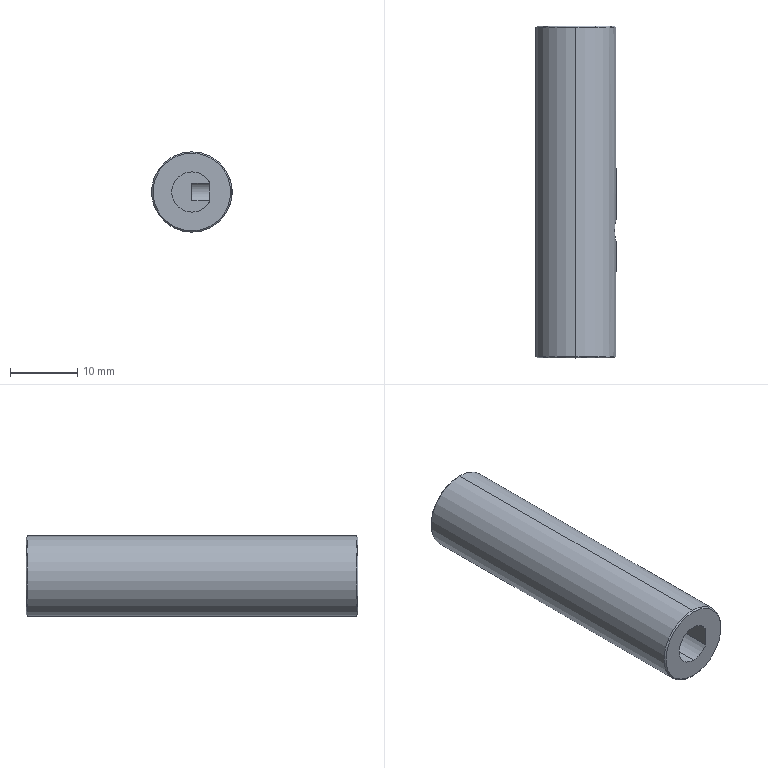Part | STEP file | 1 solid | 18 faces | box 12 x 49.5 x 12 mm | volume 5016 mm3 | cylinder 7 | plane 7 | cone 4 | commonest cylinder face diameters 6 x3 3.3 x2 12 x2